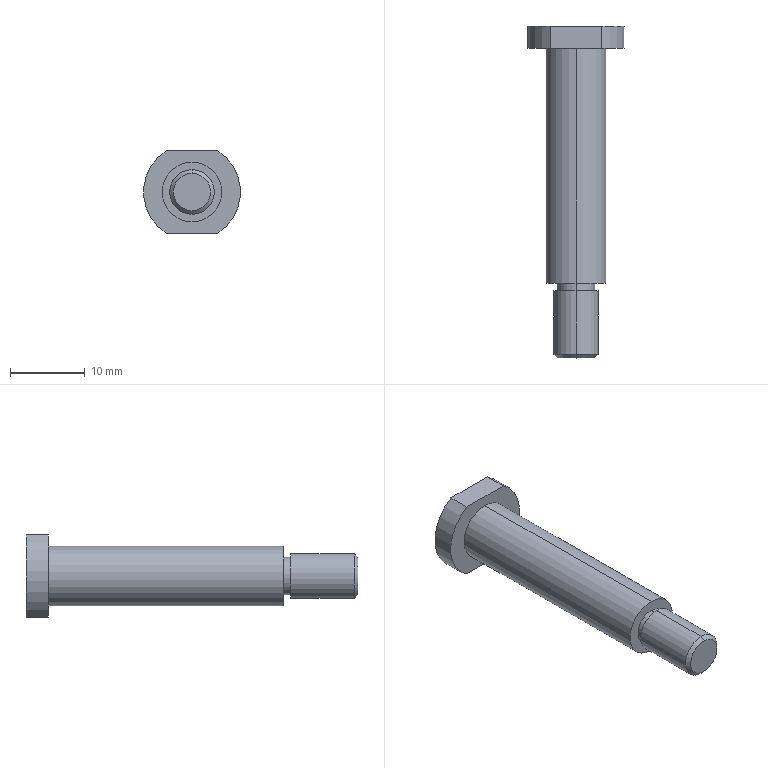Part | SolidWorks | features ICE 3, Chamfer 1, Extrusion 1, RevCut 1 | 1 solid | 17 faces | box 13 x 44.5 x 11 mm | volume 2225 mm3 | cylinder 8 | plane 7 | cone 2 | commonest cylinder face diameters 5 x2 6 x2 8 x2 13 x2
STEP:
#1=CARTESIAN_POINT('',(0.,-9.5,3.));
#2=VERTEX_POINT('',#1);
#3=CARTESIAN_POINT('',(0.,-9.5,-3.));
#4=VERTEX_POINT('',#3);
#5=CARTESIAN_POINT('',(0.,-9.5,0.));
#6=DIRECTION('',(0.,1.,0.));
#7=DIRECTION('',(0.,0.,-1.));
#8=AXIS2_PLACEMENT_3D('',#5,#6,#7);
#9=CIRCLE('',#8,3.);
#10=EDGE_CURVE('',#2,#4,#9,.T.);
#11=ORIENTED_EDGE('',*,*,#10,.T.);
#12=CARTESIAN_POINT('',(0.,-1.,-3.));
#13=VERTEX_POINT('',#12);
#14=CARTESIAN_POINT('',(0.,-10.,-3.));
#15=DIRECTION('',(0.,1.,0.));
#16=VECTOR('',#15,1000.);
#17=LINE('',#14,#16);
#18=EDGE_CURVE('',#4,#13,#17,.T.);
#19=ORIENTED_EDGE('',*,*,#18,.T.);
#20=CARTESIAN_POINT('',(0.,-1.,3.));
#21=VERTEX_POINT('',#20);
#22=CARTESIAN_POINT('',(0.,-1.,0.));
#23=DIRECTION('',(0.,1.,0.));
#24=DIRECTION('',(0.,0.,1.));
#25=AXIS2_PLACEMENT_3D('',#22,#23,#24);
#26=CIRCLE('',#25,3.);
#27=EDGE_CURVE('',#21,#13,#26,.T.);
#28=ORIENTED_EDGE('',*,*,#27,.F.);
#29=CARTESIAN_POINT('',(0.,-10.,3.));
#30=DIRECTION('',(0.,1.,0.));
#31=VECTOR('',#30,1000.);
#32=LINE('',#29,#31);
#33=EDGE_CURVE('',#2,#21,#32,.T.);
#34=ORIENTED_EDGE('',*,*,#33,.F.);
#35=EDGE_LOOP('',(#11,#19,#28,#34));
#36=FACE_OUTER_BOUND('',#35,.T.);
#37=CARTESIAN_POINT('',(0.,-10.,0.));
#38=DIRECTION('',(0.,1.,0.));
#39=DIRECTION('',(0.,0.,1.));
#40=AXIS2_PLACEMENT_3D('',#37,#38,#39);
#41=CYLINDRICAL_SURFACE('',#40,3.);
#42=ADVANCED_FACE('',(#36),#41,.T.);
#43=CARTESIAN_POINT('',(0.,-10.,-2.5));
#44=VERTEX_POINT('',#43);
#45=CARTESIAN_POINT('',(0.,-10.,2.5));
#46=VERTEX_POINT('',#45);
#47=CARTESIAN_POINT('',(0.,-10.,0.));
#48=DIRECTION('',(0.,-1.,0.));
#49=DIRECTION('',(0.,0.,-1.));
#50=AXIS2_PLACEMENT_3D('',#47,#48,#49);
#51=CIRCLE('',#50,2.5);
#52=EDGE_CURVE('',#44,#46,#51,.T.);
#53=ORIENTED_EDGE('',*,*,#52,.F.);
#54=CARTESIAN_POINT('',(0.,-10.,-2.5));
#55=DIRECTION('',(0.,0.7071,-0.7071));
#56=VECTOR('',#55,1000.);
#57=LINE('',#54,#56);
#58=EDGE_CURVE('',#44,#4,#57,.T.);
#59=ORIENTED_EDGE('',*,*,#58,.T.);
#60=ORIENTED_EDGE('',*,*,#10,.F.);
#61=CARTESIAN_POINT('',(0.,-10.,2.5));
#62=DIRECTION('',(0.,0.7071,0.7071));
#63=VECTOR('',#62,1000.);
#64=LINE('',#61,#63);
#65=EDGE_CURVE('',#46,#2,#64,.T.);
#66=ORIENTED_EDGE('',*,*,#65,.F.);
#67=EDGE_LOOP('',(#53,#59,#60,#66));
#68=FACE_OUTER_BOUND('',#67,.T.);
#69=CARTESIAN_POINT('',(0.,-10.,0.));
#70=DIRECTION('',(0.,1.,0.));
#71=DIRECTION('',(0.,0.,1.));
#72=AXIS2_PLACEMENT_3D('',#69,#70,#71);
#73=CONICAL_SURFACE('',#72,2.5,0.7854);
#74=ADVANCED_FACE('',(#68),#73,.T.);
#75=CARTESIAN_POINT('',(0.,-1.,2.5));
#76=VERTEX_POINT('',#75);
#77=CARTESIAN_POINT('',(0.,-1.,-2.5));
#78=VERTEX_POINT('',#77);
#79=CARTESIAN_POINT('',(0.,-1.,0.));
#80=DIRECTION('',(0.,1.,0.));
#81=DIRECTION('',(0.,0.,1.));
#82=AXIS2_PLACEMENT_3D('',#79,#80,#81);
#83=CIRCLE('',#82,2.5);
#84=EDGE_CURVE('',#76,#78,#83,.T.);
#85=ORIENTED_EDGE('',*,*,#84,.T.);
#86=CARTESIAN_POINT('',(0.,0.,-2.5));
#87=VERTEX_POINT('',#86);
#88=CARTESIAN_POINT('',(0.,0.,-2.5));
#89=DIRECTION('',(0.,1.,0.));
#90=VECTOR('',#89,1000.);
#91=LINE('',#88,#90);
#92=EDGE_CURVE('',#78,#87,#91,.T.);
#93=ORIENTED_EDGE('',*,*,#92,.T.);
#94=CARTESIAN_POINT('',(0.,0.,2.5));
#95=VERTEX_POINT('',#94);
#96=CARTESIAN_POINT('',(0.,0.,0.));
#97=DIRECTION('',(0.,1.,0.));
#98=DIRECTION('',(0.,0.,1.));
#99=AXIS2_PLACEMENT_3D('',#96,#97,#98);
#100=CIRCLE('',#99,2.5);
#101=EDGE_CURVE('',#95,#87,#100,.T.);
#102=ORIENTED_EDGE('',*,*,#101,.F.);
#103=CARTESIAN_POINT('',(0.,0.,2.5));
#104=DIRECTION('',(0.,1.,0.));
#105=VECTOR('',#104,1000.);
#106=LINE('',#103,#105);
#107=EDGE_CURVE('',#76,#95,#106,.T.);
#108=ORIENTED_EDGE('',*,*,#107,.F.);
#109=EDGE_LOOP('',(#85,#93,#102,#108));
#110=FACE_OUTER_BOUND('',#109,.T.);
#111=CARTESIAN_POINT('',(0.,0.,0.));
#112=DIRECTION('',(0.,1.,0.));
#113=DIRECTION('',(0.,0.,1.));
#114=AXIS2_PLACEMENT_3D('',#111,#112,#113);
#115=CYLINDRICAL_SURFACE('',#114,2.5);
#116=ADVANCED_FACE('',(#110),#115,.T.);
#117=CARTESIAN_POINT('',(0.,31.5,4.));
#118=VERTEX_POINT('',#117);
#119=CARTESIAN_POINT('',(0.,31.5,-4.));
#120=VERTEX_POINT('',#119);
#121=CARTESIAN_POINT('',(0.,31.5,0.));
#122=DIRECTION('',(0.,1.,0.));
#123=DIRECTION('',(0.,0.,1.));
#124=AXIS2_PLACEMENT_3D('',#121,#122,#123);
#125=CIRCLE('',#124,4.);
#126=EDGE_CURVE('',#118,#120,#125,.T.);
#127=ORIENTED_EDGE('',*,*,#126,.F.);
#128=CARTESIAN_POINT('',(0.,0.,4.));
#129=VERTEX_POINT('',#128);
#130=CARTESIAN_POINT('',(0.,31.5,4.));
#131=DIRECTION('',(0.,-1.,0.));
#132=VECTOR('',#131,1000.);
#133=LINE('',#130,#132);
#134=EDGE_CURVE('',#118,#129,#133,.T.);
#135=ORIENTED_EDGE('',*,*,#134,.T.);
#136=CARTESIAN_POINT('',(0.,0.,-4.));
#137=VERTEX_POINT('',#136);
#138=CARTESIAN_POINT('',(0.,0.,0.));
#139=DIRECTION('',(0.,1.,0.));
#140=DIRECTION('',(0.,0.,1.));
#141=AXIS2_PLACEMENT_3D('',#138,#139,#140);
#142=CIRCLE('',#141,4.);
#143=EDGE_CURVE('',#129,#137,#142,.T.);
#144=ORIENTED_EDGE('',*,*,#143,.T.);
#145=CARTESIAN_POINT('',(0.,31.5,-4.));
#146=DIRECTION('',(0.,-1.,0.));
#147=VECTOR('',#146,1000.);
#148=LINE('',#145,#147);
#149=EDGE_CURVE('',#120,#137,#148,.T.);
#150=ORIENTED_EDGE('',*,*,#149,.F.);
#151=EDGE_LOOP('',(#127,#135,#144,#150));
#152=FACE_OUTER_BOUND('',#151,.T.);
#153=CARTESIAN_POINT('',(0.,31.5,0.));
#154=DIRECTION('',(0.,-1.,0.));
#155=DIRECTION('',(0.,0.,-1.));
#156=AXIS2_PLACEMENT_3D('',#153,#154,#155);
#157=CYLINDRICAL_SURFACE('',#156,4.);
#158=ADVANCED_FACE('',(#152),#157,.T.);
#159=CARTESIAN_POINT('',(3.464,34.5,-5.5));
#160=VERTEX_POINT('',#159);
#161=CARTESIAN_POINT('',(3.464,31.5,-5.5));
#162=VERTEX_POINT('',#161);
#163=CARTESIAN_POINT('',(3.464,34.5,-5.5));
#164=DIRECTION('',(0.,-1.,0.));
#165=VECTOR('',#164,1000.);
#166=LINE('',#163,#165);
#167=EDGE_CURVE('',#160,#162,#166,.T.);
#168=ORIENTED_EDGE('',*,*,#167,.F.);
#169=CARTESIAN_POINT('',(3.464,34.5,5.5));
#170=VERTEX_POINT('',#169);
#171=CARTESIAN_POINT('',(0.,34.5,0.));
#172=DIRECTION('',(0.,1.,0.));
#173=DIRECTION('',(0.,0.,1.));
#174=AXIS2_PLACEMENT_3D('',#171,#172,#173);
#175=CIRCLE('',#174,6.5);
#176=EDGE_CURVE('',#170,#160,#175,.T.);
#177=ORIENTED_EDGE('',*,*,#176,.F.);
#178=CARTESIAN_POINT('',(3.464,31.5,5.5));
#179=VERTEX_POINT('',#178);
#180=CARTESIAN_POINT('',(3.464,34.5,5.5));
#181=DIRECTION('',(0.,1.,0.));
#182=VECTOR('',#181,1000.);
#183=LINE('',#180,#182);
#184=EDGE_CURVE('',#179,#170,#183,.T.);
#185=ORIENTED_EDGE('',*,*,#184,.F.);
#186=CARTESIAN_POINT('',(0.,31.5,0.));
#187=DIRECTION('',(0.,1.,0.));
#188=DIRECTION('',(0.,0.,1.));
#189=AXIS2_PLACEMENT_3D('',#186,#187,#188);
#190=CIRCLE('',#189,6.5);
#191=EDGE_CURVE('',#179,#162,#190,.T.);
#192=ORIENTED_EDGE('',*,*,#191,.T.);
#193=EDGE_LOOP('',(#168,#177,#185,#192));
#194=FACE_OUTER_BOUND('',#193,.T.);
#195=CARTESIAN_POINT('',(0.,34.5,0.));
#196=DIRECTION('',(0.,-1.,0.));
#197=DIRECTION('',(0.,0.,-1.));
#198=AXIS2_PLACEMENT_3D('',#195,#196,#197);
#199=CYLINDRICAL_SURFACE('',#198,6.5);
#200=ADVANCED_FACE('',(#194),#199,.T.);
#201=CARTESIAN_POINT('',(-3.464,31.5,-5.5));
#202=VERTEX_POINT('',#201);
#203=CARTESIAN_POINT('',(-3.464,31.5,5.5));
#204=VERTEX_POINT('',#203);
#205=CARTESIAN_POINT('',(0.,31.5,0.));
#206=DIRECTION('',(0.,1.,0.));
#207=DIRECTION('',(0.,0.,1.));
#208=AXIS2_PLACEMENT_3D('',#205,#206,#207);
#209=CIRCLE('',#208,6.5);
#210=EDGE_CURVE('',#202,#204,#209,.T.);
#211=ORIENTED_EDGE('',*,*,#210,.T.);
#212=CARTESIAN_POINT('',(-3.464,34.5,5.5));
#213=VERTEX_POINT('',#212);
#214=CARTESIAN_POINT('',(-3.464,34.5,5.5));
#215=DIRECTION('',(0.,-1.,0.));
#216=VECTOR('',#215,1000.);
#217=LINE('',#214,#216);
#218=EDGE_CURVE('',#213,#204,#217,.T.);
#219=ORIENTED_EDGE('',*,*,#218,.F.);
#220=CARTESIAN_POINT('',(-3.464,34.5,-5.5));
#221=VERTEX_POINT('',#220);
#222=CARTESIAN_POINT('',(0.,34.5,0.));
#223=DIRECTION('',(0.,1.,0.));
#224=DIRECTION('',(0.,0.,1.));
#225=AXIS2_PLACEMENT_3D('',#222,#223,#224);
#226=CIRCLE('',#225,6.5);
#227=EDGE_CURVE('',#221,#213,#226,.T.);
#228=ORIENTED_EDGE('',*,*,#227,.F.);
#229=CARTESIAN_POINT('',(-3.464,34.5,-5.5));
#230=DIRECTION('',(0.,1.,0.));
#231=VECTOR('',#230,1000.);
#232=LINE('',#229,#231);
#233=EDGE_CURVE('',#202,#221,#232,.T.);
#234=ORIENTED_EDGE('',*,*,#233,.F.);
#235=EDGE_LOOP('',(#211,#219,#228,#234));
#236=FACE_OUTER_BOUND('',#235,.T.);
#237=CARTESIAN_POINT('',(0.,34.5,0.));
#238=DIRECTION('',(0.,-1.,0.));
#239=DIRECTION('',(0.,0.,-1.));
#240=AXIS2_PLACEMENT_3D('',#237,#238,#239);
#241=CYLINDRICAL_SURFACE('',#240,6.5);
#242=ADVANCED_FACE('',(#236),#241,.T.);
#243=ORIENTED_EDGE('',*,*,#227,.T.);
#244=CARTESIAN_POINT('',(-6.5,34.5,5.5));
#245=DIRECTION('',(1.,0.,0.));
#246=VECTOR('',#245,1000.);
#247=LINE('',#244,#246);
#248=EDGE_CURVE('',#213,#170,#247,.T.);
#249=ORIENTED_EDGE('',*,*,#248,.T.);
#250=ORIENTED_EDGE('',*,*,#176,.T.);
#251=CARTESIAN_POINT('',(-6.5,34.5,-5.5));
#252=DIRECTION('',(-1.,0.,0.));
#253=VECTOR('',#252,1000.);
#254=LINE('',#251,#253);
#255=EDGE_CURVE('',#160,#221,#254,.T.);
#256=ORIENTED_EDGE('',*,*,#255,.T.);
#257=EDGE_LOOP('',(#243,#249,#250,#256));
#258=FACE_OUTER_BOUND('',#257,.T.);
#259=CARTESIAN_POINT('',(0.,34.5,0.));
#260=DIRECTION('',(0.,1.,0.));
#261=DIRECTION('',(0.,0.,1.));
#262=AXIS2_PLACEMENT_3D('',#259,#260,#261);
#263=PLANE('',#262);
#264=ADVANCED_FACE('',(#258),#263,.T.);
#265=CARTESIAN_POINT('',(0.,31.5,0.));
#266=DIRECTION('',(0.,1.,0.));
#267=DIRECTION('',(0.,0.,1.));
#268=AXIS2_PLACEMENT_3D('',#265,#266,#267);
#269=CIRCLE('',#268,4.);
#270=EDGE_CURVE('',#120,#118,#269,.T.);
#271=ORIENTED_EDGE('',*,*,#270,.T.);
#272=ORIENTED_EDGE('',*,*,#126,.T.);
#273=EDGE_LOOP('',(#271,#272));
#274=FACE_BOUND('',#273,.T.);
#275=CARTESIAN_POINT('',(0.,31.5,5.5));
#276=DIRECTION('',(1.,0.,0.));
#277=VECTOR('',#276,1000.);
#278=LINE('',#275,#277);
#279=EDGE_CURVE('',#204,#179,#278,.T.);
#280=ORIENTED_EDGE('',*,*,#279,.F.);
#281=ORIENTED_EDGE('',*,*,#210,.F.);
#282=CARTESIAN_POINT('',(0.,31.5,-5.5));
#283=DIRECTION('',(-1.,0.,0.));
#284=VECTOR('',#283,1000.);
#285=LINE('',#282,#284);
#286=EDGE_CURVE('',#162,#202,#285,.T.);
#287=ORIENTED_EDGE('',*,*,#286,.F.);
#288=ORIENTED_EDGE('',*,*,#191,.F.);
#289=EDGE_LOOP('',(#280,#281,#287,#288));
#290=FACE_OUTER_BOUND('',#289,.T.);
#291=CARTESIAN_POINT('',(0.,31.5,0.));
#292=DIRECTION('',(0.,1.,0.));
#293=DIRECTION('',(0.,0.,1.));
#294=AXIS2_PLACEMENT_3D('',#291,#292,#293);
#295=PLANE('',#294);
#296=ADVANCED_FACE('',(#274,#290),#295,.F.);
#297=ORIENTED_EDGE('',*,*,#134,.F.);
#298=ORIENTED_EDGE('',*,*,#270,.F.);
#299=ORIENTED_EDGE('',*,*,#149,.T.);
#300=CARTESIAN_POINT('',(0.,0.,0.));
#301=DIRECTION('',(0.,1.,0.));
#302=DIRECTION('',(0.,0.,1.));
#303=AXIS2_PLACEMENT_3D('',#300,#301,#302);
#304=CIRCLE('',#303,4.);
#305=EDGE_CURVE('',#137,#129,#304,.T.);
#306=ORIENTED_EDGE('',*,*,#305,.T.);
#307=EDGE_LOOP('',(#297,#298,#299,#306));
#308=FACE_OUTER_BOUND('',#307,.T.);
#309=CARTESIAN_POINT('',(0.,31.5,0.));
#310=DIRECTION('',(0.,-1.,0.));
#311=DIRECTION('',(0.,0.,-1.));
#312=AXIS2_PLACEMENT_3D('',#309,#310,#311);
#313=CYLINDRICAL_SURFACE('',#312,4.);
#314=ADVANCED_FACE('',(#308),#313,.T.);
#315=ORIENTED_EDGE('',*,*,#305,.F.);
#316=ORIENTED_EDGE('',*,*,#143,.F.);
#317=EDGE_LOOP('',(#315,#316));
#318=FACE_OUTER_BOUND('',#317,.T.);
#319=ORIENTED_EDGE('',*,*,#101,.T.);
#320=CARTESIAN_POINT('',(0.,0.,0.));
#321=DIRECTION('',(0.,1.,0.));
#322=DIRECTION('',(0.,0.,1.));
#323=AXIS2_PLACEMENT_3D('',#320,#321,#322);
#324=CIRCLE('',#323,2.5);
#325=EDGE_CURVE('',#87,#95,#324,.T.);
#326=ORIENTED_EDGE('',*,*,#325,.T.);
#327=EDGE_LOOP('',(#319,#326));
#328=FACE_BOUND('',#327,.T.);
#329=CARTESIAN_POINT('',(0.,0.,0.));
#330=DIRECTION('',(0.,1.,0.));
#331=DIRECTION('',(0.,0.,1.));
#332=AXIS2_PLACEMENT_3D('',#329,#330,#331);
#333=PLANE('',#332);
#334=ADVANCED_FACE('',(#318,#328),#333,.F.);
#335=ORIENTED_EDGE('',*,*,#167,.T.);
#336=ORIENTED_EDGE('',*,*,#286,.T.);
#337=ORIENTED_EDGE('',*,*,#233,.T.);
#338=ORIENTED_EDGE('',*,*,#255,.F.);
#339=EDGE_LOOP('',(#335,#336,#337,#338));
#340=FACE_OUTER_BOUND('',#339,.T.);
#341=CARTESIAN_POINT('',(-6.5,-10.,-5.5));
#342=DIRECTION('',(0.,0.,-1.));
#343=DIRECTION('',(-1.,0.,0.));
#344=AXIS2_PLACEMENT_3D('',#341,#342,#343);
#345=PLANE('',#344);
#346=ADVANCED_FACE('',(#340),#345,.T.);
#347=ORIENTED_EDGE('',*,*,#218,.T.);
#348=ORIENTED_EDGE('',*,*,#279,.T.);
#349=ORIENTED_EDGE('',*,*,#184,.T.);
#350=ORIENTED_EDGE('',*,*,#248,.F.);
#351=EDGE_LOOP('',(#347,#348,#349,#350));
#352=FACE_OUTER_BOUND('',#351,.T.);
#353=CARTESIAN_POINT('',(-6.5,-10.,5.5));
#354=DIRECTION('',(0.,0.,1.));
#355=DIRECTION('',(1.,0.,0.));
#356=AXIS2_PLACEMENT_3D('',#353,#354,#355);
#357=PLANE('',#356);
#358=ADVANCED_FACE('',(#352),#357,.T.);
#359=ORIENTED_EDGE('',*,*,#84,.F.);
#360=CARTESIAN_POINT('',(0.,-1.,0.));
#361=DIRECTION('',(0.,1.,0.));
#362=DIRECTION('',(0.,0.,1.));
#363=AXIS2_PLACEMENT_3D('',#360,#361,#362);
#364=CIRCLE('',#363,2.5);
#365=EDGE_CURVE('',#78,#76,#364,.T.);
#366=ORIENTED_EDGE('',*,*,#365,.F.);
#367=EDGE_LOOP('',(#359,#366));
#368=FACE_BOUND('',#367,.T.);
#369=ORIENTED_EDGE('',*,*,#27,.T.);
#370=CARTESIAN_POINT('',(0.,-1.,0.));
#371=DIRECTION('',(0.,1.,0.));
#372=DIRECTION('',(0.,0.,1.));
#373=AXIS2_PLACEMENT_3D('',#370,#371,#372);
#374=CIRCLE('',#373,3.);
#375=EDGE_CURVE('',#13,#21,#374,.T.);
#376=ORIENTED_EDGE('',*,*,#375,.T.);
#377=EDGE_LOOP('',(#369,#376));
#378=FACE_OUTER_BOUND('',#377,.T.);
#379=CARTESIAN_POINT('',(-3.,-1.,0.));
#380=DIRECTION('',(0.,-1.,0.));
#381=DIRECTION('',(0.,0.,-1.));
#382=AXIS2_PLACEMENT_3D('',#379,#380,#381);
#383=PLANE('',#382);
#384=ADVANCED_FACE('',(#368,#378),#383,.F.);
#385=ORIENTED_EDGE('',*,*,#92,.F.);
#386=ORIENTED_EDGE('',*,*,#365,.T.);
#387=ORIENTED_EDGE('',*,*,#107,.T.);
#388=ORIENTED_EDGE('',*,*,#325,.F.);
#389=EDGE_LOOP('',(#385,#386,#387,#388));
#390=FACE_OUTER_BOUND('',#389,.T.);
#391=CARTESIAN_POINT('',(0.,0.,0.));
#392=DIRECTION('',(0.,1.,0.));
#393=DIRECTION('',(0.,0.,1.));
#394=AXIS2_PLACEMENT_3D('',#391,#392,#393);
#395=CYLINDRICAL_SURFACE('',#394,2.5);
#396=ADVANCED_FACE('',(#390),#395,.T.);
#397=CARTESIAN_POINT('',(0.,-10.,0.));
#398=DIRECTION('',(0.,-1.,0.));
#399=DIRECTION('',(0.,0.,-1.));
#400=AXIS2_PLACEMENT_3D('',#397,#398,#399);
#401=CIRCLE('',#400,2.5);
#402=EDGE_CURVE('',#46,#44,#401,.T.);
#403=ORIENTED_EDGE('',*,*,#402,.T.);
#404=ORIENTED_EDGE('',*,*,#52,.T.);
#405=EDGE_LOOP('',(#403,#404));
#406=FACE_OUTER_BOUND('',#405,.T.);
#407=CARTESIAN_POINT('',(0.,-10.,0.));
#408=DIRECTION('',(0.,-1.,0.));
#409=DIRECTION('',(0.,0.,-1.));
#410=AXIS2_PLACEMENT_3D('',#407,#408,#409);
#411=PLANE('',#410);
#412=ADVANCED_FACE('',(#406),#411,.T.);
#413=ORIENTED_EDGE('',*,*,#58,.F.);
#414=ORIENTED_EDGE('',*,*,#402,.F.);
#415=ORIENTED_EDGE('',*,*,#65,.T.);
#416=CARTESIAN_POINT('',(0.,-9.5,0.));
#417=DIRECTION('',(0.,1.,0.));
#418=DIRECTION('',(0.,0.,-1.));
#419=AXIS2_PLACEMENT_3D('',#416,#417,#418);
#420=CIRCLE('',#419,3.);
#421=EDGE_CURVE('',#4,#2,#420,.T.);
#422=ORIENTED_EDGE('',*,*,#421,.F.);
#423=EDGE_LOOP('',(#413,#414,#415,#422));
#424=FACE_OUTER_BOUND('',#423,.T.);
#425=CARTESIAN_POINT('',(0.,-10.,0.));
#426=DIRECTION('',(0.,1.,0.));
#427=DIRECTION('',(0.,0.,1.));
#428=AXIS2_PLACEMENT_3D('',#425,#426,#427);
#429=CONICAL_SURFACE('',#428,2.5,0.7854);
#430=ADVANCED_FACE('',(#424),#429,.T.);
#431=ORIENTED_EDGE('',*,*,#18,.F.);
#432=ORIENTED_EDGE('',*,*,#421,.T.);
#433=ORIENTED_EDGE('',*,*,#33,.T.);
#434=ORIENTED_EDGE('',*,*,#375,.F.);
#435=EDGE_LOOP('',(#431,#432,#433,#434));
#436=FACE_OUTER_BOUND('',#435,.T.);
#437=CARTESIAN_POINT('',(0.,-10.,0.));
#438=DIRECTION('',(0.,1.,0.));
#439=DIRECTION('',(0.,0.,1.));
#440=AXIS2_PLACEMENT_3D('',#437,#438,#439);
#441=CYLINDRICAL_SURFACE('',#440,3.);
#442=ADVANCED_FACE('',(#436),#441,.T.);
#443=CLOSED_SHELL('',(#42,#74,#116,#158,#200,#242,#264,#296,#314,#334,#346,#358,#384,#396,#412,#430,#442));
#444=MANIFOLD_SOLID_BREP('',#443);
#445=CARTESIAN_POINT('',(0.,0.,0.));
#446=DIRECTION('',(0.,0.,1.));
#447=DIRECTION('',(1.,0.,0.));
#448=AXIS2_PLACEMENT_3D('',#445,#446,#447);
#449=(LENGTH_UNIT()NAMED_UNIT(*)SI_UNIT(.MILLI.,.METRE.));
#450=UNCERTAINTY_MEASURE_WITH_UNIT(LENGTH_MEASURE(0.00001),#449,'','');
#451=(NAMED_UNIT(*)PLANE_ANGLE_UNIT()SI_UNIT($,.RADIAN.));
#452=(NAMED_UNIT(*)SI_UNIT($,.STERADIAN.)SOLID_ANGLE_UNIT());
#453=(GEOMETRIC_REPRESENTATION_CONTEXT(3)GLOBAL_UNCERTAINTY_ASSIGNED_CONTEXT((#450))GLOBAL_UNIT_ASSIGNED_CONTEXT((#449,#451,#452))REPRESENTATION_CONTEXT('',''));
#454=ADVANCED_BREP_SHAPE_REPRESENTATION('',(#444,#448),#453);